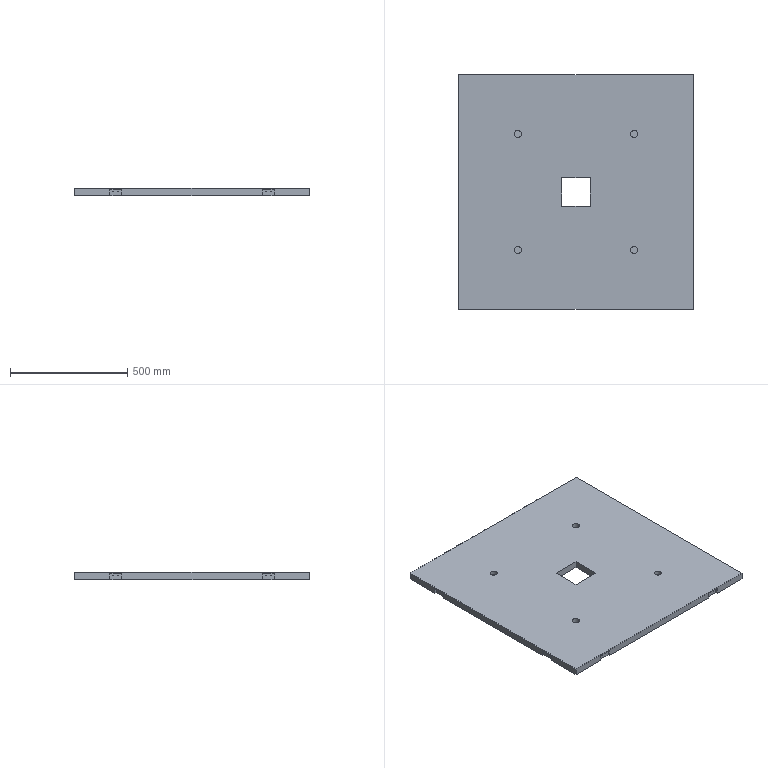Part | SolidWorks | features CirPattern 2, ICE 2, Extrusion 1, HoleWzd 1 | 1 solid | 118 faces | box 1000 x 1000 x 30 mm | volume 29440024 mm3 | plane 46 | cylinder 40 | cone 32 | commonest cylinder face diameters 3.3 x32 30 x8